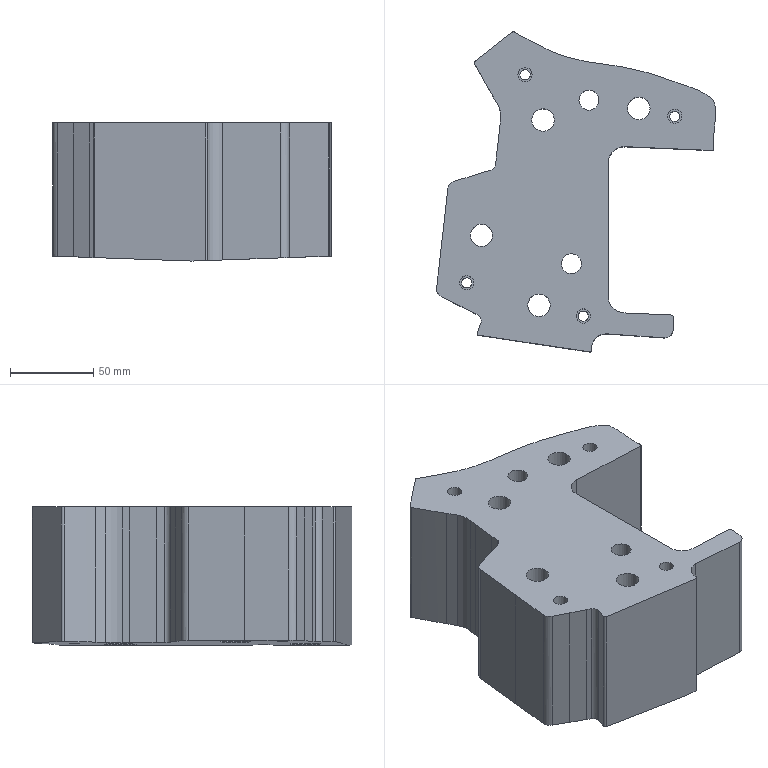Part | NX | features 8 2 | 1 solid | 82 faces | box 167.566 x 192.265 x 83 mm | volume 1361570 mm3 | cylinder 48 | plane 32 | spline 2 | commonest cylinder face diameters 20 x6 2 x5 6.2 x4 8.5 x4 13.5 x4 10 x3